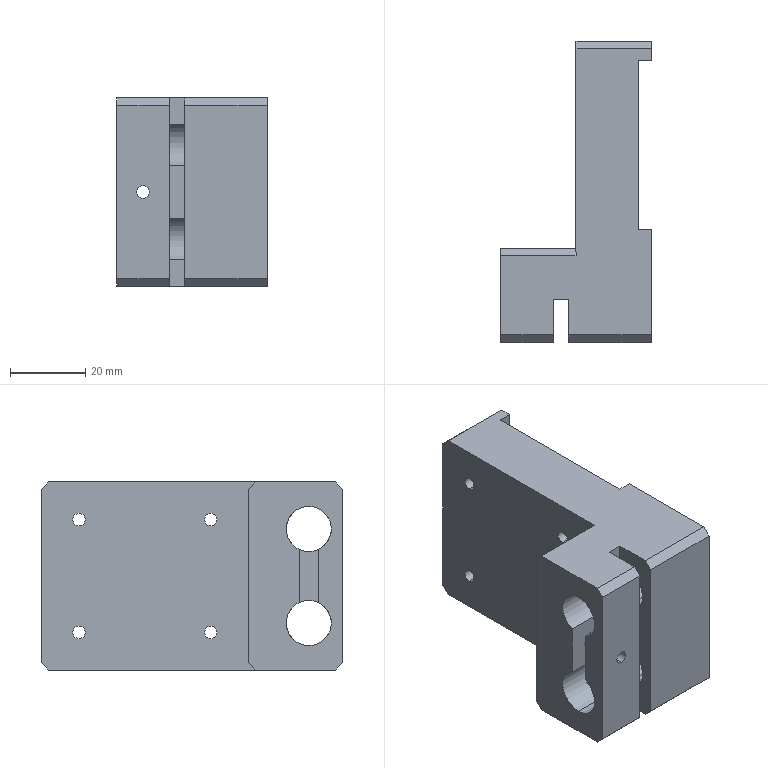Part | SolidWorks | features BaseBody 1 | 1 solid | 48 faces | box 40 x 80 x 50 mm | volume 84231 mm3 | plane 28 | cylinder 20 | commonest cylinder face diameters 3.3 x10 12 x6 4.5 x2 8 x2